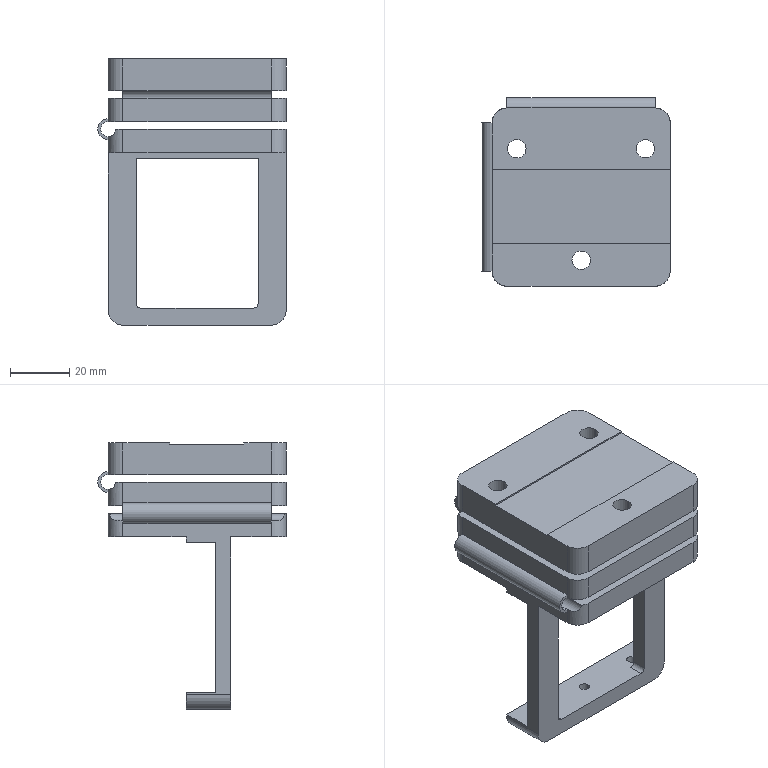Part | SolidWorks | features ICE 23, HoleWzd 2, DelFace 1, Extrusion 1, Fillet 1 | 1 solid | 94 faces | box 63.5 x 63.5 x 89.7 mm | volume 98956 mm3 | cylinder 51 | plane 37 | cone 6 | commonest cylinder face diameters 10 x14 12 x12 3.3 x6 6.2 x6 6 x4 7 x4